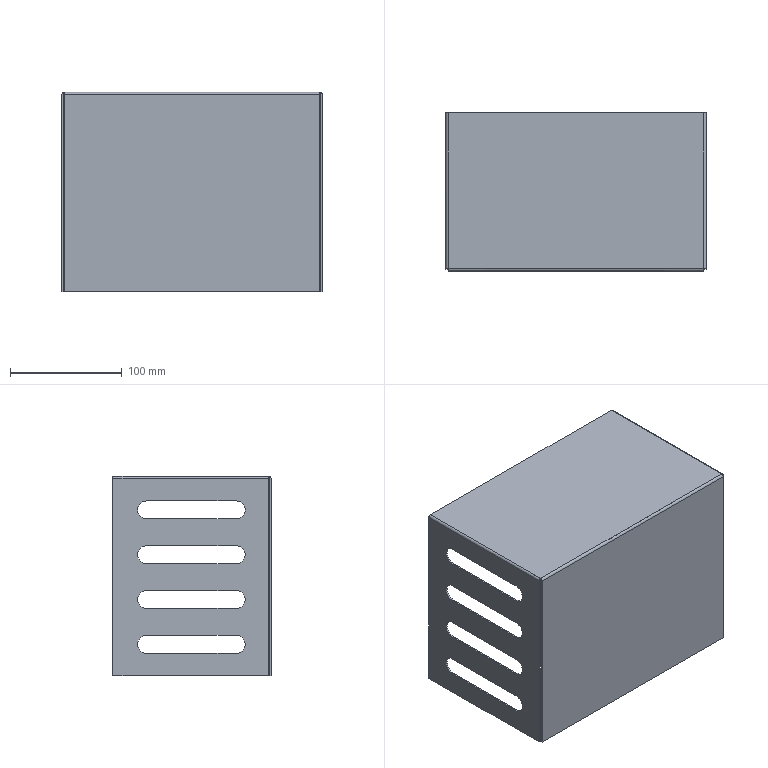Part | SolidWorks | features EdgeFlange 1, FlatPattern 1, ICE 1, LPattern 1, SMBaseFlange 1, SheetMetal 1 | 1 solid | 62 faces | box 232.4 x 141.2 x 178 mm | volume 132403 mm3 | plane 36 | cylinder 22 | spline 4 | commonest cylinder face diameters 16 x16 1.473 x3 3.873 x3